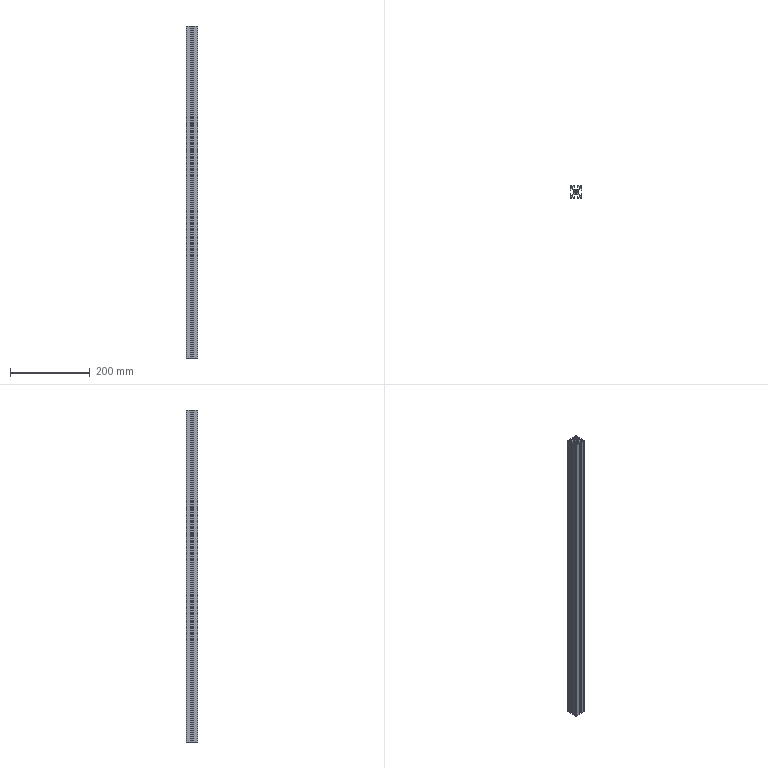Part | STEP file | SQ-8-3030W-835_Default | 1 solid | 84 faces | box 30 x 30 x 835 mm | volume 317751 mm3 | plane 62 | cylinder 22 | commonest cylinder face diameters 0.6 x8 4.2 x8 4 x4 6.8 x2